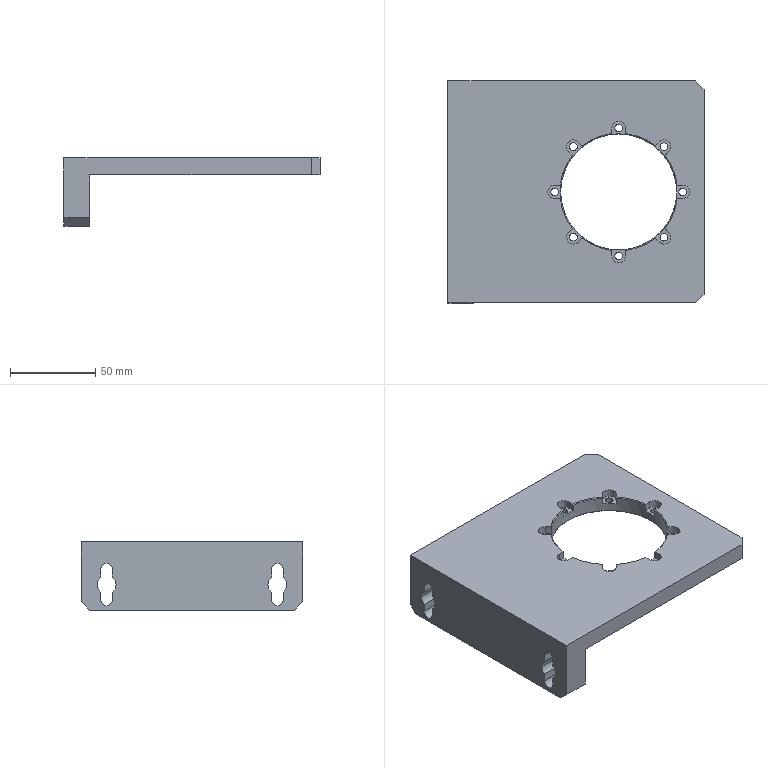NC program | NX | posted with a generic post | part box 150 x 130 x 40 mm
Whole program, first 1719 of 2019 lines:
N10 G17 G21 G94 G90
(FLOOR_WALL_COPY_COPY , TOOL : D80)
N12 T19 M6
N14 G54
N16 G17 G0 G90 X120. Y-64.997 B0. C0. S6500 M3
N18 G43 Z30. H19
N20 Z7.5
N22 G94 G1 Z4.5 F1500.
N24 X115.
N26 X-115.
N28 Y-55.429
N30 Y-15.999
N32 X115.
N34 Y33.
N36 X-115.
N38 X-120.
N40 Z7.5
N42 G0 Z30.
N44 X120. Y-64.997
N46 Z7.
N48 G1 Z4.
N50 X115.
N52 X-115.
N54 Y-55.429
N56 Y-15.999
N58 X115.
N60 Y33.
N62 X-115.
N64 X-120.
N66 Z7.
N68 G0 Z30.
N70 X120. Y-64.997
N72 Z6.5
N74 G1 Z3.5
N76 X115.
N78 X-115.
N80 Y-55.429
N82 Y-15.999
N84 X115.
N86 Y33.
N88 X-115.
N90 X-120.
N92 Z6.5
N94 G0 Z30.
N96 X120. Y-64.997
N98 Z6.
N100 G1 Z3.
N102 X115.
N104 X-115.
N106 Y-55.429
N108 Y-15.999
N110 X115.
N112 Y33.
N114 X-115.
N116 X-120.
N118 Z6.
N120 G0 Z30.
N122 X120. Y-64.997
N124 Z5.5
N126 G1 Z2.5
N128 X115.
N130 X-115.
N132 Y-55.429
N134 Y-15.999
N136 X115.
N138 Y33.
N140 X-115.
N142 X-120.
N144 Z5.5
N146 G0 Z30.
N148 X120. Y-64.997
N150 Z5.
N152 G1 Z2.
N154 X115.
N156 X-115.
N158 Y-55.429
N160 Y-15.999
N162 X115.
N164 Y33.
N166 X-115.
N168 X-120.
N170 Z5.
N172 G0 Z30.
N174 X120. Y-64.997
N176 Z4.5
N178 G1 Z1.5
N180 X115.
N182 X-115.
N184 Y-55.429
N186 Y-15.999
N188 X115.
N190 Y33.
N192 X-115.
N194 X-120.
N196 Z4.5
N198 G0 Z30.
N200 X120. Y-64.997
N202 Z4.
N204 G1 Z1.
N206 X115.
N208 X-115.
N210 Y-55.429
N212 Y-15.999
N214 X115.
N216 Y33.
N218 X-115.
N220 X-120.
N222 Z4.
N224 G0 Z30.
N226 X120. Y-64.997
N228 Z3.5
N230 G1 Z0.5
N232 X115.
N234 X-115.
N236 Y-55.429
N238 Y-15.999
N240 X115.
N242 Y33.
N244 X-115.
N246 X-120.
N248 Z3.5
N250 G0 Z30.
N252 X120. Y-64.997
N254 Z3.
N256 G1 Z0.
N258 X115.
N260 X-115.
N262 Y-55.429
N264 Y-15.999
N266 X115.
N268 Y33.
N270 X-115.
N272 X-120.
N274 Z3.
N276 G0 Z30.
N278 M5
(FLOOR_WALL , TOOL : D10)
N280 T15 M6
N282 G54
N284 G17 G0 G90 X80.5 Y73.5 B0. C0. S9500 M3
N286 G43 Z30. H15
N288 Z-11.95
N290 G94 G1 Z-14.95 F1000.
N292 Y70.5
N294 Y-70.142 F3000.
N296 G2 X80.142 Y-70.5 R0.358
N298 G1 X80.104
N300 G2 X79.704 Y-70.1 R0.4
N302 G1 Y70.142
N304 G3 X79.346 Y70.5 R0.358
N306 G1 X79.308
N308 G3 X78.908 Y70.1 R0.4
N310 G1 Y-70.142
N312 G2 X78.549 Y-70.5 R0.358
N314 G1 X78.511
N316 G2 X78.111 Y-70.1 R0.4
N318 G1 Y70.142
N320 G3 X77.753 Y70.5 R0.358
N322 G1 X77.715
N324 G3 X77.315 Y70.1 R0.4
N326 G1 Y-70.142
N328 G2 X76.957 Y-70.5 R0.358
N330 G1 X76.919
N332 G2 X76.519 Y-70.1 R0.4
N334 G1 Y70.142
N336 G3 X76.161 Y70.5 R0.358
N338 G1 X76.123
N340 G3 X75.723 Y70.1 R0.4
N342 G1 Y-70.142
N344 G2 X75.365 Y-70.5 R0.358
N346 G1 X75.327
N348 G2 X74.927 Y-70.1 R0.4
N350 G1 Y70.142
N352 G3 X74.568 Y70.5 R0.358
N354 G1 X74.531
N356 G3 X74.131 Y70.1 R0.4
N358 G1 Y-70.142
N360 G2 X73.772 Y-70.5 R0.358
N362 G1 X73.734
N364 G2 X73.334 Y-70.1 R0.4
N366 G1 Y70.142
N368 G3 X72.976 Y70.5 R0.358
N370 G1 X72.938
N372 G3 X72.538 Y70.1 R0.4
N374 G1 Y-70.142
N376 G2 X72.18 Y-70.5 R0.358
N378 G1 X72.142
N380 G2 X71.742 Y-70.1 R0.4
N382 G1 Y70.142
N384 G3 X71.384 Y70.5 R0.358
N386 G1 X71.346
N388 G3 X70.946 Y70.1 R0.4
N390 G1 Y-70.142
N392 G2 X70.588 Y-70.5 R0.358
N394 G1 X70.55
N396 G2 X70.15 Y-70.1 R0.4
N398 G1 Y70.142
N400 G3 X69.791 Y70.5 R0.358
N402 G1 X69.754
N404 G3 X69.354 Y70.1 R0.4
N406 G1 Y-70.142
N408 G2 X68.995 Y-70.5 R0.358
N410 G1 X68.957
N412 G2 X68.557 Y-70.1 R0.4
N414 G1 Y70.142
N416 G3 X68.199 Y70.5 R0.358
N418 G1 X68.161
N420 G3 X67.761 Y70.1 R0.4
N422 G1 Y-70.142
N424 G2 X67.403 Y-70.5 R0.358
N426 G1 X67.365
N428 G2 X66.965 Y-70.1 R0.4
N430 G1 Y70.142
N432 G3 X66.607 Y70.5 R0.358
N434 G1 X66.569
N436 G3 X66.169 Y70.1 R0.4
N438 G1 Y-70.142
N440 G2 X65.811 Y-70.5 R0.358
N442 G1 X65.773
N444 G2 X65.373 Y-70.1 R0.4
N446 G1 Y70.142
N448 G3 X65.014 Y70.5 R0.358
N450 G1 X64.976
N452 G3 X64.576 Y70.1 R0.4
N454 G1 Y-70.142
N456 G2 X64.218 Y-70.5 R0.358
N458 G1 X64.18
N460 G2 X63.78 Y-70.1 R0.4
N462 G1 Y70.142
N464 G3 X63.422 Y70.5 R0.358
N466 G1 X63.384
N468 G3 X62.984 Y70.1 R0.4
N470 G1 Y-70.142
N472 G2 X62.626 Y-70.5 R0.358
N474 G1 X62.588
N476 G2 X62.188 Y-70.1 R0.4
N478 G1 Y70.142
N480 G3 X61.83 Y70.5 R0.358
N482 G1 X61.792
N484 G3 X61.392 Y70.1 R0.4
N486 G1 Y-70.142
N488 G2 X61.033 Y-70.5 R0.358
N490 G1 X60.996
N492 G2 X60.596 Y-70.1 R0.4
N494 G1 Y70.142
N496 G3 X60.237 Y70.5 R0.358
N498 G1 X60.199
N500 G3 X59.799 Y70.1 R0.4
N502 G1 Y-70.142
N504 G2 X59.441 Y-70.5 R0.358
N506 G1 X59.403
N508 G2 X59.003 Y-70.1 R0.4
N510 G1 Y70.142
N512 G3 X58.645 Y70.5 R0.358
N514 G1 X58.607
N516 G3 X58.207 Y70.1 R0.4
N518 G1 Y-70.142
N520 G2 X57.849 Y-70.5 R0.358
N522 G1 X57.811
N524 G2 X57.411 Y-70.1 R0.4
N526 G1 Y70.142
N528 G3 X57.053 Y70.5 R0.358
N530 G1 X57.015
N532 G3 X56.615 Y70.1 R0.4
N534 G1 Y-70.142
N536 G2 X56.256 Y-70.5 R0.358
N538 G1 X56.219
N540 G2 X55.819 Y-70.1 R0.4
N542 G1 Y70.142
N544 G3 X55.46 Y70.5 R0.358
N546 G1 X55.422
N548 G3 X55.022 Y70.1 R0.4
N550 G1 Y-70.142
N552 G2 X54.664 Y-70.5 R0.358
N554 G1 X54.626
N556 G2 X54.226 Y-70.1 R0.4
N558 G1 Y70.142
N560 G3 X53.868 Y70.5 R0.358
N562 G1 X53.83
N564 G3 X53.43 Y70.1 R0.4
N566 G1 Y-70.142
N568 G2 X53.072 Y-70.5 R0.358
N570 G1 X53.034
N572 G2 X52.634 Y-70.1 R0.4
N574 G1 Y70.142
N576 G3 X52.276 Y70.5 R0.358
N578 G1 X52.238
N580 G3 X51.838 Y70.1 R0.4
N582 G1 Y-70.142
N584 G2 X51.479 Y-70.5 R0.358
N586 G1 X51.441
N588 G2 X51.041 Y-70.1 R0.4
N590 G1 Y70.142
N592 G3 X50.683 Y70.5 R0.358
N594 G1 X50.645
N596 G3 X50.245 Y70.1 R0.4
N598 G1 Y-70.142
N600 G2 X49.887 Y-70.5 R0.358
N602 G1 X49.849
N604 G2 X49.449 Y-70.1 R0.4
N606 G1 Y70.142
N608 G3 X49.091 Y70.5 R0.358
N610 G1 X49.053
N612 G3 X48.653 Y70.1 R0.4
N614 G1 Y-70.142
N616 G2 X48.295 Y-70.5 R0.358
N618 G1 X48.257
N620 G2 X47.857 Y-70.1 R0.4
N622 G1 Y70.142
N624 G3 X47.498 Y70.5 R0.358
N626 G1 X47.461
N628 G3 X47.061 Y70.1 R0.4
N630 G1 Y-70.142
N632 G2 X46.702 Y-70.5 R0.358
N634 G1 X46.664
N636 G2 X46.264 Y-70.1 R0.4
N638 G1 Y70.142
N640 G3 X45.906 Y70.5 R0.358
N642 G1 X45.868
N644 G3 X45.468 Y70.1 R0.4
N646 G1 Y-70.142
N648 G2 X45.11 Y-70.5 R0.358
N650 G1 X45.072
N652 G2 X44.672 Y-70.1 R0.4
N654 G1 Y70.142
N656 G3 X44.314 Y70.5 R0.358
N658 G1 X44.276
N660 G3 X43.876 Y70.1 R0.4
N662 G1 Y-70.142
N664 G2 X43.518 Y-70.5 R0.358
N666 G1 X43.48
N668 G2 X43.08 Y-70.1 R0.4
N670 G1 Y70.142
N672 G3 X42.721 Y70.5 R0.358
N674 G1 X42.684
N676 G3 X42.284 Y70.1 R0.4
N678 G1 Y-70.142
N680 G2 X41.925 Y-70.5 R0.358
N682 G1 X41.887
N684 G2 X41.487 Y-70.1 R0.4
N686 G1 Y70.142
N688 G3 X41.129 Y70.5 R0.358
N690 G1 X41.091
N692 G3 X40.691 Y70.1 R0.4
N694 G1 Y-70.142
N696 G2 X40.333 Y-70.5 R0.358
N698 G1 X40.295
N700 G2 X39.895 Y-70.1 R0.4
N702 G1 Y70.142
N704 G3 X39.537 Y70.5 R0.358
N706 G1 X39.499
N708 G3 X39.099 Y70.1 R0.4
N710 G1 Y-70.142
N712 G2 X38.741 Y-70.5 R0.358
N714 G1 X38.703
N716 G2 X38.303 Y-70.1 R0.4
N718 G1 Y70.142
N720 G3 X37.944 Y70.5 R0.358
N722 G1 X37.906
N724 G3 X37.506 Y70.1 R0.4
N726 G1 Y-70.142
N728 G2 X37.148 Y-70.5 R0.358
N730 G1 X37.11
N732 G2 X36.71 Y-70.1 R0.4
N734 G1 Y70.142
N736 G3 X36.352 Y70.5 R0.358
N738 G1 X36.314
N740 G3 X35.914 Y70.1 R0.4
N742 G1 Y-70.142
N744 G2 X35.556 Y-70.5 R0.358
N746 G1 X35.518
N748 G2 X35.118 Y-70.1 R0.4
N750 G1 Y70.142
N752 G3 X34.76 Y70.5 R0.358
N754 G1 X34.722
N756 G3 X34.322 Y70.1 R0.4
N758 G1 Y-70.142
N760 G2 X33.963 Y-70.5 R0.358
N762 G1 X33.926
N764 G2 X33.526 Y-70.1 R0.4
N766 G1 Y70.142
N768 G3 X33.167 Y70.5 R0.358
N770 G1 X33.129
N772 G3 X32.729 Y70.1 R0.4
N774 G1 Y-70.142
N776 G2 X32.371 Y-70.5 R0.358
N778 G1 X32.333
N780 G2 X31.933 Y-70.1 R0.4
N782 G1 Y70.142
N784 G3 X31.575 Y70.5 R0.358
N786 G1 X31.537
N788 G3 X31.137 Y70.1 R0.4
N790 G1 Y-70.142
N792 G2 X30.779 Y-70.5 R0.358
N794 G1 X30.741
N796 G2 X30.341 Y-70.1 R0.4
N798 G1 Y70.142
N800 G3 X29.983 Y70.5 R0.358
N802 G1 X29.945
N804 G3 X29.545 Y70.1 R0.4
N806 G1 Y-70.142
N808 G2 X29.186 Y-70.5 R0.358
N810 G1 X29.149
N812 G2 X28.749 Y-70.1 R0.4
N814 G1 Y70.142
N816 G3 X28.39 Y70.5 R0.358
N818 G1 X28.352
N820 G3 X27.952 Y70.1 R0.4
N822 G1 Y-70.142
N824 G2 X27.594 Y-70.5 R0.358
N826 G1 X27.556
N828 G2 X27.156 Y-70.1 R0.4
N830 G1 Y70.142
N832 G3 X26.798 Y70.5 R0.358
N834 G1 X26.76
N836 G3 X26.36 Y70.1 R0.4
N838 G1 Y-70.142
N840 G2 X26.002 Y-70.5 R0.358
N842 G1 X25.964
N844 G2 X25.564 Y-70.1 R0.4
N846 G1 Y70.142
N848 G3 X25.206 Y70.5 R0.358
N850 G1 X25.168
N852 G3 X24.768 Y70.1 R0.4
N854 G1 Y-70.142
N856 G2 X24.409 Y-70.5 R0.358
N858 G1 X24.371
N860 G2 X23.971 Y-70.1 R0.4
N862 G1 Y70.142
N864 G3 X23.613 Y70.5 R0.358
N866 G1 X23.575
N868 G3 X23.175 Y70.1 R0.4
N870 G1 Y-70.142
N872 G2 X22.817 Y-70.5 R0.358
N874 G1 X22.779
N876 G2 X22.379 Y-70.1 R0.4
N878 G1 Y70.142
N880 G3 X22.021 Y70.5 R0.358
N882 G1 X21.983
N884 G3 X21.583 Y70.1 R0.4
N886 G1 Y-70.142
N888 G2 X21.225 Y-70.5 R0.358
N890 G1 X21.187
N892 G2 X20.787 Y-70.1 R0.4
N894 G1 Y70.142
N896 G3 X20.428 Y70.5 R0.358
N898 G1 X20.391
N900 G3 X19.991 Y70.1 R0.4
N902 G1 Y-70.142
N904 G2 X19.632 Y-70.5 R0.358
N906 G1 X19.594
N908 G2 X19.194 Y-70.1 R0.4
N910 G1 Y70.142
N912 G3 X18.836 Y70.5 R0.358
N914 G1 X18.798
N916 G3 X18.398 Y70.1 R0.4
N918 G1 Y-70.142
N920 G2 X18.04 Y-70.5 R0.358
N922 G1 X18.002
N924 G2 X17.602 Y-70.1 R0.4
N926 G1 Y70.142
N928 G3 X17.244 Y70.5 R0.358
N930 G1 X17.206
N932 G3 X16.806 Y70.1 R0.4
N934 G1 Y-70.142
N936 G2 X16.448 Y-70.5 R0.358
N938 G1 X16.41
N940 G2 X16.01 Y-70.1 R0.4
N942 G1 Y70.142
N944 G3 X15.651 Y70.5 R0.358
N946 G1 X15.614
N948 G3 X15.214 Y70.1 R0.4
N950 G1 Y-70.142
N952 G2 X14.855 Y-70.5 R0.358
N954 G1 X14.817
N956 G2 X14.417 Y-70.1 R0.4
N958 G1 Y70.142
N960 G3 X14.059 Y70.5 R0.358
N962 G1 X14.021
N964 G3 X13.621 Y70.1 R0.4
N966 G1 Y-70.142
N968 G2 X13.263 Y-70.5 R0.358
N970 G1 X13.225
N972 G2 X12.825 Y-70.1 R0.4
N974 G1 Y70.142
N976 G3 X12.467 Y70.5 R0.358
N978 G1 X12.429
N980 G3 X12.029 Y70.1 R0.4
N982 G1 Y-70.142
N984 G2 X11.671 Y-70.5 R0.358
N986 G1 X11.633
N988 G2 X11.233 Y-70.1 R0.4
N990 G1 Y70.142
N992 G3 X10.874 Y70.5 R0.358
N994 G1 X10.836
N996 G3 X10.436 Y70.1 R0.4
N998 G1 Y-70.142
N1000 G2 X10.078 Y-70.5 R0.358
N1002 G1 X10.04
N1004 G2 X9.64 Y-70.1 R0.4
N1006 G1 Y70.142
N1008 G3 X9.282 Y70.5 R0.358
N1010 G1 X9.244
N1012 G3 X8.844 Y70.1 R0.4
N1014 G1 Y-70.142
N1016 G2 X8.486 Y-70.5 R0.358
N1018 G1 X8.448
N1020 G2 X8.048 Y-70.1 R0.4
N1022 G1 Y70.142
N1024 G3 X7.69 Y70.5 R0.358
N1026 G1 X7.652
N1028 G3 X7.252 Y70.1 R0.4
N1030 G1 Y-70.142
N1032 G2 X6.893 Y-70.5 R0.358
N1034 G1 X6.856
N1036 G2 X6.456 Y-70.1 R0.4
N1038 G1 Y70.142
N1040 G3 X6.097 Y70.5 R0.358
N1042 G1 X6.059
N1044 G3 X5.659 Y70.1 R0.4
N1046 G1 Y-70.142
N1048 G2 X5.301 Y-70.5 R0.358
N1050 G1 X5.263
N1052 G2 X4.863 Y-70.1 R0.4
N1054 G1 Y70.142
N1056 G3 X4.505 Y70.5 R0.358
N1058 G1 X4.467
N1060 G3 X4.067 Y70.1 R0.4
N1062 G1 Y-70.142
N1064 G2 X3.709 Y-70.5 R0.358
N1066 G1 X3.671
N1068 G2 X3.271 Y-70.1 R0.4
N1070 G1 Y70.142
N1072 G3 X2.913 Y70.5 R0.358
N1074 G1 X2.875
N1076 G3 X2.475 Y70.1 R0.4
N1078 G1 Y-70.142
N1080 G2 X2.116 Y-70.5 R0.358
N1082 G1 X2.079
N1084 G2 X1.679 Y-70.1 R0.4
N1086 G1 Y70.142
N1088 G3 X1.32 Y70.5 R0.358
N1090 G1 X1.282
N1092 G3 X0.882 Y70.1 R0.4
N1094 G1 Y-70.142
N1096 G2 X0.524 Y-70.5 R0.358
N1098 G1 X0.486
N1100 G2 X0.086 Y-70.1 R0.4
N1102 G1 Y70.142
N1104 G3 X-0.272 Y70.5 R0.358
N1106 G1 X-0.31
N1108 G3 X-0.71 Y70.1 R0.4
N1110 G1 Y-70.142
N1112 G2 X-1.068 Y-70.5 R0.358
N1114 G1 X-1.106
N1116 G2 X-1.506 Y-70.1 R0.4
N1118 G1 Y70.142
N1120 G3 X-1.864 Y70.5 R0.358
N1122 G1 X-1.902
N1124 G3 X-2.302 Y70.1 R0.4
N1126 G1 Y-70.142
N1128 G2 X-2.661 Y-70.5 R0.358
N1130 G1 X-2.699
N1132 G2 X-3.099 Y-70.1 R0.4
N1134 G1 Y70.142
N1136 G3 X-3.457 Y70.5 R0.358
N1138 G1 X-3.495
N1140 G3 X-3.895 Y70.1 R0.4
N1142 G1 Y-70.142
N1144 G2 X-4.253 Y-70.5 R0.358
N1146 G1 X-4.291
N1148 G2 X-4.691 Y-70.1 R0.4
N1150 G1 Y70.142
N1152 G3 X-5.049 Y70.5 R0.358
N1154 G1 X-5.087
N1156 G3 X-5.487 Y70.1 R0.4
N1158 G1 Y-70.142
N1160 G2 X-5.845 Y-70.5 R0.358
N1162 G1 X-5.883
N1164 G2 X-6.283 Y-70.1 R0.4
N1166 G1 Y70.142
N1168 G3 X-6.642 Y70.5 R0.358
N1170 G1 X-6.679
N1172 G3 X-7.079 Y70.1 R0.4
N1174 G1 Y-70.142
N1176 G2 X-7.438 Y-70.5 R0.358
N1178 G1 X-7.476
N1180 G2 X-7.876 Y-70.1 R0.4
N1182 G1 Y70.142
N1184 G3 X-8.234 Y70.5 R0.358
N1186 G1 X-8.272
N1188 G3 X-8.672 Y70.1 R0.4
N1190 G1 Y-70.142
N1192 G2 X-9.03 Y-70.5 R0.358
N1194 G1 X-9.068
N1196 G2 X-9.468 Y-70.1 R0.4
N1198 G1 Y70.142
N1200 G3 X-9.826 Y70.5 R0.358
N1202 G1 X-9.864
N1204 G3 X-10.264 Y70.1 R0.4
N1206 G1 Y-70.142
N1208 G2 X-10.622 Y-70.5 R0.358
N1210 G1 X-10.66
N1212 G2 X-11.06 Y-70.1 R0.4
N1214 G1 Y70.142
N1216 G3 X-11.419 Y70.5 R0.358
N1218 G1 X-11.456
N1220 G3 X-11.856 Y70.1 R0.4
N1222 G1 Y-70.142
N1224 G2 X-12.215 Y-70.5 R0.358
N1226 G1 X-12.253
N1228 G2 X-12.653 Y-70.1 R0.4
N1230 G1 Y70.142
N1232 G3 X-13.011 Y70.5 R0.358
N1234 G1 X-13.049
N1236 G3 X-13.449 Y70.1 R0.4
N1238 G1 Y-70.142
N1240 G2 X-13.807 Y-70.5 R0.358
N1242 G1 X-13.845
N1244 G2 X-14.245 Y-70.1 R0.4
N1246 G1 Y70.142
N1248 G3 X-14.603 Y70.5 R0.358
N1250 G1 X-14.641
N1252 G3 X-15.041 Y70.1 R0.4
N1254 G1 Y-70.142
N1256 G2 X-15.399 Y-70.5 R0.358
N1258 G1 X-15.437
N1260 G2 X-15.837 Y-70.1 R0.4
N1262 G1 Y70.142
N1264 G3 X-16.196 Y70.5 R0.358
N1266 G1 X-16.234
N1268 G3 X-16.634 Y70.1 R0.4
N1270 G1 Y-70.142
N1272 G2 X-16.992 Y-70.5 R0.358
N1274 G1 X-17.03
N1276 G2 X-17.43 Y-70.1 R0.4
N1278 G1 Y70.142
N1280 G3 X-17.788 Y70.5 R0.358
N1282 G1 X-17.826
N1284 G3 X-18.226 Y70.1 R0.4
N1286 G1 Y-70.142
N1288 G2 X-18.584 Y-70.5 R0.358
N1290 G1 X-18.622
N1292 G2 X-19.022 Y-70.1 R0.4
N1294 G1 Y70.142
N1296 G3 X-19.38 Y70.5 R0.358
N1298 G1 X-19.418
N1300 G3 X-19.818 Y70.1 R0.4
N1302 G1 Y-70.142
N1304 G2 X-20.177 Y-70.5 R0.358
N1306 G1 X-20.214
N1308 G2 X-20.614 Y-70.1 R0.4
N1310 G1 Y70.142
N1312 G3 X-20.973 Y70.5 R0.358
N1314 G1 X-21.011
N1316 G3 X-21.411 Y70.1 R0.4
N1318 G1 Y-70.142
N1320 G2 X-21.769 Y-70.5 R0.358
N1322 G1 X-21.807
N1324 G2 X-22.207 Y-70.1 R0.4
N1326 G1 Y70.142
N1328 G3 X-22.565 Y70.5 R0.358
N1330 G1 X-22.603
N1332 G3 X-23.003 Y70.1 R0.4
N1334 G1 Y-70.142
N1336 G2 X-23.361 Y-70.5 R0.358
N1338 G1 X-23.399
N1340 G2 X-23.799 Y-70.1 R0.4
N1342 G1 Y70.142
N1344 G3 X-24.157 Y70.5 R0.358
N1346 G1 X-24.195
N1348 G3 X-24.595 Y70.1 R0.4
N1350 G1 Y-70.142
N1352 G2 X-24.954 Y-70.5 R0.358
N1354 G1 X-24.991
N1356 G2 X-25.391 Y-70.1 R0.4
N1358 G1 Y70.142
N1360 G3 X-25.75 Y70.5 R0.358
N1362 G1 X-25.788
N1364 G3 X-26.188 Y70.1 R0.4
N1366 G1 Y-70.142
N1368 G2 X-26.546 Y-70.5 R0.358
N1370 G1 X-26.584
N1372 G2 X-26.984 Y-70.1 R0.4
N1374 G1 Y70.142
N1376 G3 X-27.342 Y70.5 R0.358
N1378 G1 X-27.38
N1380 G3 X-27.78 Y70.1 R0.4
N1382 G1 Y-70.142
N1384 G2 X-28.138 Y-70.5 R0.358
N1386 G1 X-28.176
N1388 G2 X-28.576 Y-70.1 R0.4
N1390 G1 Y70.142
N1392 G3 X-28.934 Y70.5 R0.358
N1394 G1 X-28.972
N1396 G3 X-29.372 Y70.1 R0.4
N1398 G1 Y-70.142
N1400 G2 X-29.731 Y-70.5 R0.358
N1402 G1 X-29.769
N1404 G2 X-30.169 Y-70.1 R0.4
N1406 G1 Y70.142
N1408 G3 X-30.527 Y70.5 R0.358
N1410 G1 X-30.565
N1412 G3 X-30.965 Y70.1 R0.4
N1414 G1 Y-70.142
N1416 G2 X-31.323 Y-70.5 R0.358
N1418 G1 X-31.361
N1420 G2 X-31.761 Y-70.1 R0.4
N1422 G1 Y70.142
N1424 G3 X-32.119 Y70.5 R0.358
N1426 G1 X-32.157
N1428 G3 X-32.557 Y70.1 R0.4
N1430 G1 Y-70.142
N1432 G2 X-32.915 Y-70.5 R0.358
N1434 G1 X-32.953
N1436 G2 X-33.353 Y-70.1 R0.4
N1438 G1 Y70.142
N1440 G3 X-33.712 Y70.5 R0.358
N1442 G1 X-33.749
N1444 G3 X-34.149 Y70.1 R0.4
N1446 G1 Y-70.142
N1448 G2 X-34.508 Y-70.5 R0.358
N1450 G1 X-34.546
N1452 G2 X-34.946 Y-70.1 R0.4
N1454 G1 Y70.142
N1456 G3 X-35.304 Y70.5 R0.358
N1458 G1 X-35.342
N1460 G3 X-35.742 Y70.1 R0.4
N1462 G1 Y-70.142
N1464 G2 X-36.1 Y-70.5 R0.358
N1466 G1 X-36.138
N1468 G2 X-36.538 Y-70.1 R0.4
N1470 G1 Y70.142
N1472 G3 X-36.896 Y70.5 R0.358
N1474 G1 X-36.934
N1476 G3 X-37.334 Y70.1 R0.4
N1478 G1 Y-70.142
N1480 G2 X-37.692 Y-70.5 R0.358
N1482 G1 X-37.73
N1484 G2 X-38.13 Y-70.1 R0.4
N1486 G1 Y70.142
N1488 G3 X-38.489 Y70.5 R0.358
N1490 G1 X-38.526
N1492 G3 X-38.926 Y70.1 R0.4
N1494 G1 Y-70.142
N1496 G2 X-39.285 Y-70.5 R0.358
N1498 G1 X-39.323
N1500 G2 X-39.723 Y-70.1 R0.4
N1502 G1 Y70.142
N1504 G3 X-40.081 Y70.5 R0.358
N1506 G1 X-40.119
N1508 G3 X-40.519 Y70.1 R0.4
N1510 G1 Y-70.142
N1512 G2 X-40.877 Y-70.5 R0.358
N1514 G1 X-40.915
N1516 G2 X-41.315 Y-70.1 R0.4
N1518 G1 Y70.142
N1520 G3 X-41.673 Y70.5 R0.358
N1522 G1 X-41.711
N1524 G3 X-42.111 Y70.1 R0.4
N1526 G1 Y-70.142
N1528 G2 X-42.469 Y-70.5 R0.358
N1530 G1 X-42.507
N1532 G2 X-42.907 Y-70.1 R0.4
N1534 G1 Y70.142
N1536 G3 X-43.266 Y70.5 R0.358
N1538 G1 X-43.304
N1540 G3 X-43.704 Y70.1 R0.4
N1542 G1 Y-70.142
N1544 G2 X-44.062 Y-70.5 R0.358
N1546 G1 X-44.1
N1548 G2 X-44.5 Y-70.1 R0.4
N1550 G1 Y70.142
N1552 G3 X-44.858 Y70.5 R0.358
N1554 G1 X-44.896
N1556 G3 X-45.296 Y70.1 R0.4
N1558 G1 Y-70.142
N1560 G2 X-45.654 Y-70.5 R0.358
N1562 G1 X-45.692
N1564 G2 X-46.092 Y-70.1 R0.4
N1566 G1 Y70.142
N1568 G3 X-46.45 Y70.5 R0.358
N1570 G1 X-46.488
N1572 G3 X-46.888 Y70.1 R0.4
N1574 G1 Y-70.142
N1576 G2 X-47.247 Y-70.5 R0.358
N1578 G1 X-47.284
N1580 G2 X-47.684 Y-70.1 R0.4
N1582 G1 Y70.142
N1584 G3 X-48.043 Y70.5 R0.358
N1586 G1 X-48.081
N1588 G3 X-48.481 Y70.1 R0.4
N1590 G1 Y-70.142
N1592 G2 X-48.839 Y-70.5 R0.358
N1594 G1 X-48.877
N1596 G2 X-49.277 Y-70.1 R0.4
N1598 G1 Y70.142
N1600 G3 X-49.635 Y70.5 R0.358
N1602 G1 X-49.673
N1604 G3 X-50.073 Y70.1 R0.4
N1606 G1 Y-70.142
N1608 G2 X-50.431 Y-70.5 R0.358
N1610 G1 X-50.469
N1612 G2 X-50.869 Y-70.1 R0.4
N1614 G1 Y70.142
N1616 G3 X-51.227 Y70.5 R0.358
N1618 G1 X-51.265
N1620 G3 X-51.665 Y70.1 R0.4
N1622 G1 Y-70.142
N1624 G2 X-52.024 Y-70.5 R0.358
N1626 G1 X-52.061
N1628 G2 X-52.461 Y-70.1 R0.4
N1630 G1 Y70.142
N1632 G3 X-52.82 Y70.5 R0.358
N1634 G1 X-52.858
N1636 G3 X-53.258 Y70.1 R0.4
N1638 G1 Y-70.142
N1640 G2 X-53.616 Y-70.5 R0.358
N1642 G1 X-53.654
N1644 G2 X-54.054 Y-70.1 R0.4
N1646 G1 Y70.142
N1648 G3 X-54.412 Y70.5 R0.358
N1650 G1 X-54.45
N1652 G3 X-54.85 Y70.1 R0.4
N1654 G1 Y-70.5
N1656 Y-73.5
N1658 Z-11.95
N1660 G0 Z30.
N1662 X80.5 Y73.5
N1664 Z-26.9
N1666 G1 Z-29.9 F1000.
N1668 Y70.5
N1670 Y-70.142 F3000.
N1672 G2 X80.142 Y-70.5 R0.358
N1674 G1 X80.104
N1676 G2 X79.704 Y-70.1 R0.4
N1678 G1 Y70.142
N1680 G3 X79.346 Y70.5 R0.358
N1682 G1 X79.308
N1684 G3 X78.908 Y70.1 R0.4
N1686 G1 Y-70.142
N1688 G2 X78.549 Y-70.5 R0.358
N1690 G1 X78.511
N1692 G2 X78.111 Y-70.1 R0.4
N1694 G1 Y70.142
N1696 G3 X77.753 Y70.5 R0.358
N1698 G1 X77.715
N1700 G3 X77.315 Y70.1 R0.4
N1702 G1 Y-70.142
N1704 G2 X76.957 Y-70.5 R0.358
N1706 G1 X76.919
N1708 G2 X76.519 Y-70.1 R0.4
N1710 G1 Y70.142
N1712 G3 X76.161 Y70.5 R0.358
N1714 G1 X76.123
N1716 G3 X75.723 Y70.1 R0.4
N1718 G1 Y-70.142
N1720 G2 X75.365 Y-70.5 R0.358
N1722 G1 X75.327
N1724 G2 X74.927 Y-70.1 R0.4
N1726 G1 Y70.142
N1728 G3 X74.568 Y70.5 R0.358
N1730 G1 X74.531
N1732 G3 X74.131 Y70.1 R0.4
N1734 G1 Y-70.142
N1736 G2 X73.772 Y-70.5 R0.358
N1738 G1 X73.734
N1740 G2 X73.334 Y-70.1 R0.4
N1742 G1 Y70.142
N1744 G3 X72.976 Y70.5 R0.358
N1746 G1 X72.938
N1748 G3 X72.538 Y70.1 R0.4
N1750 G1 Y-70.142
N1752 G2 X72.18 Y-70.5 R0.358
N1754 G1 X72.142
N1756 G2 X71.742 Y-70.1 R0.4
N1758 G1 Y70.142
N1760 G3 X71.384 Y70.5 R0.358
N1762 G1 X71.346
N1764 G3 X70.946 Y70.1 R0.4
N1766 G1 Y-70.142
N1768 G2 X70.588 Y-70.5 R0.358
N1770 G1 X70.55
N1772 G2 X70.15 Y-70.1 R0.4
N1774 G1 Y70.142
N1776 G3 X69.791 Y70.5 R0.358
N1778 G1 X69.754
N1780 G3 X69.354 Y70.1 R0.4
N1782 G1 Y-70.142
N1784 G2 X68.995 Y-70.5 R0.358
N1786 G1 X68.957
N1788 G2 X68.557 Y-70.1 R0.4
N1790 G1 Y70.142
N1792 G3 X68.199 Y70.5 R0.358
N1794 G1 X68.161
N1796 G3 X67.761 Y70.1 R0.4
N1798 G1 Y-70.142
N1800 G2 X67.403 Y-70.5 R0.358
N1802 G1 X67.365
N1804 G2 X66.965 Y-70.1 R0.4
N1806 G1 Y70.142
N1808 G3 X66.607 Y70.5 R0.358
N1810 G1 X66.569
N1812 G3 X66.169 Y70.1 R0.4
N1814 G1 Y-70.142
N1816 G2 X65.811 Y-70.5 R0.358
N1818 G1 X65.773
N1820 G2 X65.373 Y-70.1 R0.4
N1822 G1 Y70.142
N1824 G3 X65.014 Y70.5 R0.358
N1826 G1 X64.976
N1828 G3 X64.576 Y70.1 R0.4
N1830 G1 Y-70.142
N1832 G2 X64.218 Y-70.5 R0.358
N1834 G1 X64.18
N1836 G2 X63.78 Y-70.1 R0.4
N1838 G1 Y70.142
N1840 G3 X63.422 Y70.5 R0.358
N1842 G1 X63.384
N1844 G3 X62.984 Y70.1 R0.4
N1846 G1 Y-70.142
N1848 G2 X62.626 Y-70.5 R0.358
N1850 G1 X62.588
N1852 G2 X62.188 Y-70.1 R0.4
N1854 G1 Y70.142
N1856 G3 X61.83 Y70.5 R0.358
N1858 G1 X61.792
N1860 G3 X61.392 Y70.1 R0.4
N1862 G1 Y-70.142
N1864 G2 X61.033 Y-70.5 R0.358
N1866 G1 X60.996
N1868 G2 X60.596 Y-70.1 R0.4
N1870 G1 Y70.142
N1872 G3 X60.237 Y70.5 R0.358
N1874 G1 X60.199
N1876 G3 X59.799 Y70.1 R0.4
N1878 G1 Y-70.142
N1880 G2 X59.441 Y-70.5 R0.358
N1882 G1 X59.403
N1884 G2 X59.003 Y-70.1 R0.4
N1886 G1 Y70.142
N1888 G3 X58.645 Y70.5 R0.358
N1890 G1 X58.607
N1892 G3 X58.207 Y70.1 R0.4
N1894 G1 Y-70.142
N1896 G2 X57.849 Y-70.5 R0.358
N1898 G1 X57.811
N1900 G2 X57.411 Y-70.1 R0.4
N1902 G1 Y70.142
N1904 G3 X57.053 Y70.5 R0.358
N1906 G1 X57.015
N1908 G3 X56.615 Y70.1 R0.4
N1910 G1 Y-70.142
N1912 G2 X56.256 Y-70.5 R0.358
N1914 G1 X56.219
N1916 G2 X55.819 Y-70.1 R0.4
N1918 G1 Y70.142
N1920 G3 X55.46 Y70.5 R0.358
N1922 G1 X55.422
N1924 G3 X55.022 Y70.1 R0.4
N1926 G1 Y-70.142
N1928 G2 X54.664 Y-70.5 R0.358
N1930 G1 X54.626
N1932 G2 X54.226 Y-70.1 R0.4
N1934 G1 Y70.142
N1936 G3 X53.868 Y70.5 R0.358
N1938 G1 X53.83
N1940 G3 X53.43 Y70.1 R0.4
N1942 G1 Y-70.142
N1944 G2 X53.072 Y-70.5 R0.358
N1946 G1 X53.034
N1948 G2 X52.634 Y-70.1 R0.4
N1950 G1 Y70.142
N1952 G3 X52.276 Y70.5 R0.358
N1954 G1 X52.238
N1956 G3 X51.838 Y70.1 R0.4
N1958 G1 Y-70.142
N1960 G2 X51.479 Y-70.5 R0.358
N1962 G1 X51.441
N1964 G2 X51.041 Y-70.1 R0.4
N1966 G1 Y70.142
N1968 G3 X50.683 Y70.5 R0.358
N1970 G1 X50.645
N1972 G3 X50.245 Y70.1 R0.4
N1974 G1 Y-70.142
N1976 G2 X49.887 Y-70.5 R0.358
N1978 G1 X49.849
N1980 G2 X49.449 Y-70.1 R0.4
N1982 G1 Y70.142
N1984 G3 X49.091 Y70.5 R0.358
N1986 G1 X49.053
N1988 G3 X48.653 Y70.1 R0.4
N1990 G1 Y-70.142
N1992 G2 X48.295 Y-70.5 R0.358
N1994 G1 X48.257
N1996 G2 X47.857 Y-70.1 R0.4
N1998 G1 Y70.142
N2000 G3 X47.498 Y70.5 R0.358
N2002 G1 X47.461
N2004 G3 X47.061 Y70.1 R0.4
N2006 G1 Y-70.142
N2008 G2 X46.702 Y-70.5 R0.358
N2010 G1 X46.664
N2012 G2 X46.264 Y-70.1 R0.4
N2014 G1 Y70.142
N2016 G3 X45.906 Y70.5 R0.358
N2018 G1 X45.868
N2020 G3 X45.468 Y70.1 R0.4
N2022 G1 Y-70.142
N2024 G2 X45.11 Y-70.5 R0.358
N2026 G1 X45.072
N2028 G2 X44.672 Y-70.1 R0.4
N2030 G1 Y70.142
N2032 G3 X44.314 Y70.5 R0.358
N2034 G1 X44.276
N2036 G3 X43.876 Y70.1 R0.4
N2038 G1 Y-70.142
N2040 G2 X43.518 Y-70.5 R0.358
N2042 G1 X43.48
N2044 G2 X43.08 Y-70.1 R0.4
N2046 G1 Y70.142
N2048 G3 X42.721 Y70.5 R0.358
N2050 G1 X42.684
N2052 G3 X42.284 Y70.1 R0.4
N2054 G1 Y-70.142
N2056 G2 X41.925 Y-70.5 R0.358
N2058 G1 X41.887
N2060 G2 X41.487 Y-70.1 R0.4
N2062 G1 Y70.142
N2064 G3 X41.129 Y70.5 R0.358
N2066 G1 X41.091
N2068 G3 X40.691 Y70.1 R0.4
N2070 G1 Y-70.142
N2072 G2 X40.333 Y-70.5 R0.358
N2074 G1 X40.295
N2076 G2 X39.895 Y-70.1 R0.4
N2078 G1 Y70.142
N2080 G3 X39.537 Y70.5 R0.358
N2082 G1 X39.499
N2084 G3 X39.099 Y70.1 R0.4
N2086 G1 Y-70.142
N2088 G2 X38.741 Y-70.5 R0.358
N2090 G1 X38.703
N2092 G2 X38.303 Y-70.1 R0.4
N2094 G1 Y70.142
N2096 G3 X37.944 Y70.5 R0.358
N2098 G1 X37.906
N2100 G3 X37.506 Y70.1 R0.4
N2102 G1 Y-70.142
N2104 G2 X37.148 Y-70.5 R0.358
N2106 G1 X37.11
N2108 G2 X36.71 Y-70.1 R0.4
N2110 G1 Y70.142
N2112 G3 X36.352 Y70.5 R0.358
N2114 G1 X36.314
N2116 G3 X35.914 Y70.1 R0.4
N2118 G1 Y-70.142
N2120 G2 X35.556 Y-70.5 R0.358
N2122 G1 X35.518
N2124 G2 X35.118 Y-70.1 R0.4
N2126 G1 Y70.142
N2128 G3 X34.76 Y70.5 R0.358
N2130 G1 X34.722
N2132 G3 X34.322 Y70.1 R0.4
N2134 G1 Y-70.142
N2136 G2 X33.963 Y-70.5 R0.358
N2138 G1 X33.926
N2140 G2 X33.526 Y-70.1 R0.4
N2142 G1 Y70.142
N2144 G3 X33.167 Y70.5 R0.358
N2146 G1 X33.129
N2148 G3 X32.729 Y70.1 R0.4
N2150 G1 Y-70.142
N2152 G2 X32.371 Y-70.5 R0.358
N2154 G1 X32.333
N2156 G2 X31.933 Y-70.1 R0.4
N2158 G1 Y70.142
N2160 G3 X31.575 Y70.5 R0.358
N2162 G1 X31.537
N2164 G3 X31.137 Y70.1 R0.4
N2166 G1 Y-70.142
N2168 G2 X30.779 Y-70.5 R0.358
N2170 G1 X30.741
N2172 G2 X30.341 Y-70.1 R0.4
N2174 G1 Y70.142
N2176 G3 X29.983 Y70.5 R0.358
N2178 G1 X29.945
N2180 G3 X29.545 Y70.1 R0.4
N2182 G1 Y-70.142
N2184 G2 X29.186 Y-70.5 R0.358
N2186 G1 X29.149
N2188 G2 X28.749 Y-70.1 R0.4
N2190 G1 Y70.142
N2192 G3 X28.39 Y70.5 R0.358
N2194 G1 X28.352
N2196 G3 X27.952 Y70.1 R0.4
N2198 G1 Y-70.142
N2200 G2 X27.594 Y-70.5 R0.358
N2202 G1 X27.556
N2204 G2 X27.156 Y-70.1 R0.4
N2206 G1 Y70.142
N2208 G3 X26.798 Y70.5 R0.358
N2210 G1 X26.76
N2212 G3 X26.36 Y70.1 R0.4
N2214 G1 Y-70.142
N2216 G2 X26.002 Y-70.5 R0.358
N2218 G1 X25.964
N2220 G2 X25.564 Y-70.1 R0.4
N2222 G1 Y70.142
N2224 G3 X25.206 Y70.5 R0.358
N2226 G1 X25.168
N2228 G3 X24.768 Y70.1 R0.4
N2230 G1 Y-70.142
N2232 G2 X24.409 Y-70.5 R0.358
N2234 G1 X24.371
N2236 G2 X23.971 Y-70.1 R0.4
N2238 G1 Y70.142
N2240 G3 X23.613 Y70.5 R0.358
N2242 G1 X23.575
N2244 G3 X23.175 Y70.1 R0.4
N2246 G1 Y-70.142
N2248 G2 X22.817 Y-70.5 R0.358
N2250 G1 X22.779
N2252 G2 X22.379 Y-70.1 R0.4
N2254 G1 Y70.142
N2256 G3 X22.021 Y70.5 R0.358
N2258 G1 X21.983
N2260 G3 X21.583 Y70.1 R0.4
N2262 G1 Y-70.142
N2264 G2 X21.225 Y-70.5 R0.358
N2266 G1 X21.187
N2268 G2 X20.787 Y-70.1 R0.4
N2270 G1 Y70.142
N2272 G3 X20.428 Y70.5 R0.358
N2274 G1 X20.391
N2276 G3 X19.991 Y70.1 R0.4
N2278 G1 Y-70.142
N2280 G2 X19.632 Y-70.5 R0.358
N2282 G1 X19.594
N2284 G2 X19.194 Y-70.1 R0.4
N2286 G1 Y70.142
N2288 G3 X18.836 Y70.5 R0.358
N2290 G1 X18.798
N2292 G3 X18.398 Y70.1 R0.4
N2294 G1 Y-70.142
N2296 G2 X18.04 Y-70.5 R0.358
N2298 G1 X18.002
N2300 G2 X17.602 Y-70.1 R0.4
N2302 G1 Y70.142
N2304 G3 X17.244 Y70.5 R0.358
N2306 G1 X17.206
N2308 G3 X16.806 Y70.1 R0.4
N2310 G1 Y-70.142
N2312 G2 X16.448 Y-70.5 R0.358
N2314 G1 X16.41
N2316 G2 X16.01 Y-70.1 R0.4
N2318 G1 Y70.142
N2320 G3 X15.651 Y70.5 R0.358
N2322 G1 X15.614
N2324 G3 X15.214 Y70.1 R0.4
N2326 G1 Y-70.142
N2328 G2 X14.855 Y-70.5 R0.358
N2330 G1 X14.817
N2332 G2 X14.417 Y-70.1 R0.4
N2334 G1 Y70.142
N2336 G3 X14.059 Y70.5 R0.358
N2338 G1 X14.021
N2340 G3 X13.621 Y70.1 R0.4
N2342 G1 Y-70.142
N2344 G2 X13.263 Y-70.5 R0.358
N2346 G1 X13.225
N2348 G2 X12.825 Y-70.1 R0.4
N2350 G1 Y70.142
N2352 G3 X12.467 Y70.5 R0.358
N2354 G1 X12.429
N2356 G3 X12.029 Y70.1 R0.4
N2358 G1 Y-70.142
N2360 G2 X11.671 Y-70.5 R0.358
N2362 G1 X11.633
N2364 G2 X11.233 Y-70.1 R0.4
N2366 G1 Y70.142
N2368 G3 X10.874 Y70.5 R0.358
N2370 G1 X10.836
N2372 G3 X10.436 Y70.1 R0.4
N2374 G1 Y-70.142
N2376 G2 X10.078 Y-70.5 R0.358
N2378 G1 X10.04
N2380 G2 X9.64 Y-70.1 R0.4
N2382 G1 Y70.142
N2384 G3 X9.282 Y70.5 R0.358
N2386 G1 X9.244
N2388 G3 X8.844 Y70.1 R0.4
N2390 G1 Y-70.142
N2392 G2 X8.486 Y-70.5 R0.358
N2394 G1 X8.448
N2396 G2 X8.048 Y-70.1 R0.4
N2398 G1 Y70.142
N2400 G3 X7.69 Y70.5 R0.358
N2402 G1 X7.652
N2404 G3 X7.252 Y70.1 R0.4
N2406 G1 Y-70.142
N2408 G2 X6.893 Y-70.5 R0.358
N2410 G1 X6.856
N2412 G2 X6.456 Y-70.1 R0.4
N2414 G1 Y70.142
N2416 G3 X6.097 Y70.5 R0.358
N2418 G1 X6.059
N2420 G3 X5.659 Y70.1 R0.4
N2422 G1 Y-70.142
N2424 G2 X5.301 Y-70.5 R0.358
N2426 G1 X5.263
N2428 G2 X4.863 Y-70.1 R0.4
N2430 G1 Y70.142
N2432 G3 X4.505 Y70.5 R0.358
N2434 G1 X4.467
N2436 G3 X4.067 Y70.1 R0.4
N2438 G1 Y-70.142
N2440 G2 X3.709 Y-70.5 R0.358
N2442 G1 X3.671
N2444 G2 X3.271 Y-70.1 R0.4
N2446 G1 Y70.142
N2448 G3 X2.913 Y70.5 R0.358
N2450 G1 X2.875
N2452 G3 X2.475 Y70.1 R0.4
N2454 G1 Y-70.142
N2456 G2 X2.116 Y-70.5 R0.358
N2458 G1 X2.079
N2460 G2 X1.679 Y-70.1 R0.4
N2462 G1 Y70.142
N2464 G3 X1.32 Y70.5 R0.358
N2466 G1 X1.282
N2468 G3 X0.882 Y70.1 R0.4
N2470 G1 Y-70.142
N2472 G2 X0.524 Y-70.5 R0.358
N2474 G1 X0.486
N2476 G2 X0.086 Y-70.1 R0.4
N2478 G1 Y70.142
N2480 G3 X-0.272 Y70.5 R0.358
N2482 G1 X-0.31
N2484 G3 X-0.71 Y70.1 R0.4
N2486 G1 Y-70.142
N2488 G2 X-1.068 Y-70.5 R0.358
N2490 G1 X-1.106
N2492 G2 X-1.506 Y-70.1 R0.4
N2494 G1 Y70.142
N2496 G3 X-1.864 Y70.5 R0.358
N2498 G1 X-1.902
N2500 G3 X-2.302 Y70.1 R0.4
N2502 G1 Y-70.142
N2504 G2 X-2.661 Y-70.5 R0.358
N2506 G1 X-2.699
N2508 G2 X-3.099 Y-70.1 R0.4
N2510 G1 Y70.142
N2512 G3 X-3.457 Y70.5 R0.358
N2514 G1 X-3.495
N2516 G3 X-3.895 Y70.1 R0.4
N2518 G1 Y-70.142
N2520 G2 X-4.253 Y-70.5 R0.358
N2522 G1 X-4.291
N2524 G2 X-4.691 Y-70.1 R0.4
N2526 G1 Y70.142
N2528 G3 X-5.049 Y70.5 R0.358
N2530 G1 X-5.087
N2532 G3 X-5.487 Y70.1 R0.4
N2534 G1 Y-70.142
N2536 G2 X-5.845 Y-70.5 R0.358
N2538 G1 X-5.883
N2540 G2 X-6.283 Y-70.1 R0.4
N2542 G1 Y70.142
N2544 G3 X-6.642 Y70.5 R0.358
N2546 G1 X-6.679
N2548 G3 X-7.079 Y70.1 R0.4
N2550 G1 Y-70.142
N2552 G2 X-7.438 Y-70.5 R0.358
N2554 G1 X-7.476
N2556 G2 X-7.876 Y-70.1 R0.4
N2558 G1 Y70.142
N2560 G3 X-8.234 Y70.5 R0.358
N2562 G1 X-8.272
N2564 G3 X-8.672 Y70.1 R0.4
N2566 G1 Y-70.142
N2568 G2 X-9.03 Y-70.5 R0.358
N2570 G1 X-9.068
N2572 G2 X-9.468 Y-70.1 R0.4
N2574 G1 Y70.142
N2576 G3 X-9.826 Y70.5 R0.358
N2578 G1 X-9.864
N2580 G3 X-10.264 Y70.1 R0.4
N2582 G1 Y-70.142
N2584 G2 X-10.622 Y-70.5 R0.358
N2586 G1 X-10.66
N2588 G2 X-11.06 Y-70.1 R0.4
N2590 G1 Y70.142
N2592 G3 X-11.419 Y70.5 R0.358
N2594 G1 X-11.456
N2596 G3 X-11.856 Y70.1 R0.4
N2598 G1 Y-70.142
N2600 G2 X-12.215 Y-70.5 R0.358
N2602 G1 X-12.253
N2604 G2 X-12.653 Y-70.1 R0.4
N2606 G1 Y70.142
N2608 G3 X-13.011 Y70.5 R0.358
N2610 G1 X-13.049
N2612 G3 X-13.449 Y70.1 R0.4
N2614 G1 Y-70.142
N2616 G2 X-13.807 Y-70.5 R0.358
N2618 G1 X-13.845
N2620 G2 X-14.245 Y-70.1 R0.4
N2622 G1 Y70.142
N2624 G3 X-14.603 Y70.5 R0.358
N2626 G1 X-14.641
N2628 G3 X-15.041 Y70.1 R0.4
N2630 G1 Y-70.142
N2632 G2 X-15.399 Y-70.5 R0.358
N2634 G1 X-15.437
N2636 G2 X-15.837 Y-70.1 R0.4
N2638 G1 Y70.142
N2640 G3 X-16.196 Y70.5 R0.358
N2642 G1 X-16.234
N2644 G3 X-16.634 Y70.1 R0.4
N2646 G1 Y-70.142
N2648 G2 X-16.992 Y-70.5 R0.358
N2650 G1 X-17.03
N2652 G2 X-17.43 Y-70.1 R0.4
N2654 G1 Y70.142
N2656 G3 X-17.788 Y70.5 R0.358
N2658 G1 X-17.826
N2660 G3 X-18.226 Y70.1 R0.4
N2662 G1 Y-70.142
N2664 G2 X-18.584 Y-70.5 R0.358
N2666 G1 X-18.622
N2668 G2 X-19.022 Y-70.1 R0.4
N2670 G1 Y70.142
N2672 G3 X-19.38 Y70.5 R0.358
N2674 G1 X-19.418
N2676 G3 X-19.818 Y70.1 R0.4
N2678 G1 Y-70.142
N2680 G2 X-20.177 Y-70.5 R0.358
N2682 G1 X-20.214
N2684 G2 X-20.614 Y-70.1 R0.4
N2686 G1 Y70.142
N2688 G3 X-20.973 Y70.5 R0.358
N2690 G1 X-21.011
N2692 G3 X-21.411 Y70.1 R0.4
N2694 G1 Y-70.142
N2696 G2 X-21.769 Y-70.5 R0.358
N2698 G1 X-21.807
N2700 G2 X-22.207 Y-70.1 R0.4
N2702 G1 Y70.142
N2704 G3 X-22.565 Y70.5 R0.358
N2706 G1 X-22.603
N2708 G3 X-23.003 Y70.1 R0.4
N2710 G1 Y-70.142
N2712 G2 X-23.361 Y-70.5 R0.358
N2714 G1 X-23.399
N2716 G2 X-23.799 Y-70.1 R0.4
N2718 G1 Y70.142
N2720 G3 X-24.157 Y70.5 R0.358
N2722 G1 X-24.195
N2724 G3 X-24.595 Y70.1 R0.4
N2726 G1 Y-70.142
N2728 G2 X-24.954 Y-70.5 R0.358
N2730 G1 X-24.991
N2732 G2 X-25.391 Y-70.1 R0.4
N2734 G1 Y70.142
N2736 G3 X-25.75 Y70.5 R0.358
N2738 G1 X-25.788
N2740 G3 X-26.188 Y70.1 R0.4
N2742 G1 Y-70.142
N2744 G2 X-26.546 Y-70.5 R0.358
N2746 G1 X-26.584
N2748 G2 X-26.984 Y-70.1 R0.4
N2750 G1 Y70.142
N2752 G3 X-27.342 Y70.5 R0.358
N2754 G1 X-27.38
N2756 G3 X-27.78 Y70.1 R0.4
N2758 G1 Y-70.142
N2760 G2 X-28.138 Y-70.5 R0.358
N2762 G1 X-28.176
N2764 G2 X-28.576 Y-70.1 R0.4
N2766 G1 Y70.142
N2768 G3 X-28.934 Y70.5 R0.358
N2770 G1 X-28.972
N2772 G3 X-29.372 Y70.1 R0.4
N2774 G1 Y-70.142
N2776 G2 X-29.731 Y-70.5 R0.358
N2778 G1 X-29.769
N2780 G2 X-30.169 Y-70.1 R0.4
N2782 G1 Y70.142
N2784 G3 X-30.527 Y70.5 R0.358
N2786 G1 X-30.565
N2788 G3 X-30.965 Y70.1 R0.4
N2790 G1 Y-70.142
N2792 G2 X-31.323 Y-70.5 R0.358
N2794 G1 X-31.361
N2796 G2 X-31.761 Y-70.1 R0.4
N2798 G1 Y70.142
N2800 G3 X-32.119 Y70.5 R0.358
N2802 G1 X-32.157
N2804 G3 X-32.557 Y70.1 R0.4
N2806 G1 Y-70.142
N2808 G2 X-32.915 Y-70.5 R0.358
N2810 G1 X-32.953
N2812 G2 X-33.353 Y-70.1 R0.4
N2814 G1 Y70.142
N2816 G3 X-33.712 Y70.5 R0.358
N2818 G1 X-33.749
N2820 G3 X-34.149 Y70.1 R0.4
N2822 G1 Y-70.142
N2824 G2 X-34.508 Y-70.5 R0.358
N2826 G1 X-34.546
N2828 G2 X-34.946 Y-70.1 R0.4
N2830 G1 Y70.142
N2832 G3 X-35.304 Y70.5 R0.358
N2834 G1 X-35.342
N2836 G3 X-35.742 Y70.1 R0.4
N2838 G1 Y-70.142
N2840 G2 X-36.1 Y-70.5 R0.358
N2842 G1 X-36.138
N2844 G2 X-36.538 Y-70.1 R0.4
N2846 G1 Y70.142
N2848 G3 X-36.896 Y70.5 R0.358
N2850 G1 X-36.934
N2852 G3 X-37.334 Y70.1 R0.4
N2854 G1 Y-70.142
N2856 G2 X-37.692 Y-70.5 R0.358
N2858 G1 X-37.73
N2860 G2 X-38.13 Y-70.1 R0.4
N2862 G1 Y70.142
N2864 G3 X-38.489 Y70.5 R0.358
N2866 G1 X-38.526
N2868 G3 X-38.926 Y70.1 R0.4
N2870 G1 Y-70.142
N2872 G2 X-39.285 Y-70.5 R0.358
N2874 G1 X-39.323
N2876 G2 X-39.723 Y-70.1 R0.4
N2878 G1 Y70.142
N2880 G3 X-40.081 Y70.5 R0.358
N2882 G1 X-40.119
N2884 G3 X-40.519 Y70.1 R0.4
N2886 G1 Y-70.142
N2888 G2 X-40.877 Y-70.5 R0.358
N2890 G1 X-40.915
N2892 G2 X-41.315 Y-70.1 R0.4
N2894 G1 Y70.142
N2896 G3 X-41.673 Y70.5 R0.358
N2898 G1 X-41.711
N2900 G3 X-42.111 Y70.1 R0.4
N2902 G1 Y-70.142
N2904 G2 X-42.469 Y-70.5 R0.358
N2906 G1 X-42.507
N2908 G2 X-42.907 Y-70.1 R0.4
N2910 G1 Y70.142
N2912 G3 X-43.266 Y70.5 R0.358
N2914 G1 X-43.304
N2916 G3 X-43.704 Y70.1 R0.4
N2918 G1 Y-70.142
N2920 G2 X-44.062 Y-70.5 R0.358
N2922 G1 X-44.1
N2924 G2 X-44.5 Y-70.1 R0.4
N2926 G1 Y70.142
N2928 G3 X-44.858 Y70.5 R0.358
N2930 G1 X-44.896
N2932 G3 X-45.296 Y70.1 R0.4
N2934 G1 Y-70.142
N2936 G2 X-45.654 Y-70.5 R0.358
N2938 G1 X-45.692
N2940 G2 X-46.092 Y-70.1 R0.4
N2942 G1 Y70.142
N2944 G3 X-46.45 Y70.5 R0.358
N2946 G1 X-46.488
N2948 G3 X-46.888 Y70.1 R0.4
N2950 G1 Y-70.142
N2952 G2 X-47.247 Y-70.5 R0.358
N2954 G1 X-47.284
N2956 G2 X-47.684 Y-70.1 R0.4
N2958 G1 Y70.142
N2960 G3 X-48.043 Y70.5 R0.358
N2962 G1 X-48.081
N2964 G3 X-48.481 Y70.1 R0.4
N2966 G1 Y-70.142
N2968 G2 X-48.839 Y-70.5 R0.358
N2970 G1 X-48.877
N2972 G2 X-49.277 Y-70.1 R0.4
N2974 G1 Y70.142
N2976 G3 X-49.635 Y70.5 R0.358
N2978 G1 X-49.673
N2980 G3 X-50.073 Y70.1 R0.4
N2982 G1 Y-70.142
N2984 G2 X-50.431 Y-70.5 R0.358
N2986 G1 X-50.469
N2988 G2 X-50.869 Y-70.1 R0.4
N2990 G1 Y70.142
N2992 G3 X-51.227 Y70.5 R0.358
N2994 G1 X-51.265
N2996 G3 X-51.665 Y70.1 R0.4
N2998 G1 Y-70.142
N3000 G2 X-52.024 Y-70.5 R0.358
N3002 G1 X-52.061
N3004 G2 X-52.461 Y-70.1 R0.4
N3006 G1 Y70.142
N3008 G3 X-52.82 Y70.5 R0.358
N3010 G1 X-52.858
N3012 G3 X-53.258 Y70.1 R0.4
N3014 G1 Y-70.142
N3016 G2 X-53.616 Y-70.5 R0.358
N3018 G1 X-53.654
N3020 G2 X-54.054 Y-70.1 R0.4
N3022 G1 Y70.142
N3024 G3 X-54.412 Y70.5 R0.358
N3026 G1 X-54.45
N3028 G3 X-54.85 Y70.1 R0.4
N3030 G1 Y-70.5
N3032 Y-73.5
N3034 Z-26.9
N3036 G0 Z30.
N3038 M5
(FLOOR_WALL_COPY_1 , TOOL : D10JING)
N3040 T14 M6
N3042 G54
N3044 G17 G0 G90 X-55. Y73. B0. C0. S9500 M3
N3046 G43 Z30. H14
N3048 Z-11.95
N3050 G94 G1 Z-14.95 F1000.
N3052 Y70.
N3054 Y-70. F1200.
N3056 Y-73.
N3058 Z-11.95
N3060 G0 Z30.
N3062 Y73.
N3064 Z-26.9
N3066 G1 Z-29.9 F1000.
N3068 Y70.
N3070 Y-70. F1200.
N3072 Y-73.
N3074 Z-26.9
N3076 G0 Z30.
(FLOOR_WALL_COPY_1_COPY , TOOL : D10JING)
N3078 X80. Y73.
N3080 Z-27.
N3082 G1 Z-30. F1000.
N3084 Y70.
N3086 Y-67.758 F1200.
N3088 G2 X77.758 Y-70. R2.242
N3090 G1 X77.519
N3092 G2 X75.019 Y-67.5 R2.5
N3094 G1 Y67.758
N3096 G3 X72.777 Y70. R2.242
N3098 G1 X72.537
N3100 G3 X70.037 Y67.5 R2.5
N3102 G1 Y-67.758
N3104 G2 X67.795 Y-70. R2.242
N3106 G1 X67.556
N3108 G2 X65.056 Y-67.5 R2.5
N3110 G1 Y67.758
N3112 G3 X62.814 Y70. R2.242
N3114 G1 X62.574
N3116 G3 X60.074 Y67.5 R2.5
N3118 G1 Y-67.758
N3120 G2 X57.832 Y-70. R2.242
N3122 G1 X57.593
N3124 G2 X55.093 Y-67.5 R2.5
N3126 G1 Y67.758
N3128 G3 X52.851 Y70. R2.242
N3130 G1 X52.611
N3132 G3 X50.111 Y67.5 R2.5
N3134 G1 Y-67.758
N3136 G2 X47.869 Y-70. R2.242
N3138 G1 X47.63
N3140 G2 X45.13 Y-67.5 R2.5
N3142 G1 Y67.758
N3144 G3 X42.888 Y70. R2.242
N3146 G1 X42.648
N3148 G3 X40.148 Y67.5 R2.5
N3150 G1 Y-67.758
N3152 G2 X37.906 Y-70. R2.242
N3154 G1 X37.667
N3156 G2 X35.167 Y-67.5 R2.5
N3158 G1 Y67.758
N3160 G3 X32.925 Y70. R2.242
N3162 G1 X32.685
N3164 G3 X30.185 Y67.5 R2.5
N3166 G1 Y-67.758
N3168 G2 X27.944 Y-70. R2.242
N3170 G1 X27.704
N3172 G2 X25.204 Y-67.5 R2.5
N3174 G1 Y67.758
N3176 G3 X22.962 Y70. R2.242
N3178 G1 X22.722
N3180 G3 X20.222 Y67.5 R2.5
N3182 G1 Y-67.758
N3184 G2 X17.981 Y-70. R2.242
N3186 G1 X17.741
N3188 G2 X15.241 Y-67.5 R2.5
N3190 G1 Y67.758
N3192 G3 X12.999 Y70. R2.242
N3194 G1 X12.759
N3196 G3 X10.259 Y67.5 R2.5
N3198 G1 Y-67.758
N3200 G2 X8.018 Y-70. R2.242
N3202 G1 X7.778
N3204 G2 X5.278 Y-67.5 R2.5
N3206 G1 Y67.509
N3208 G3 X2.787 Y70. R2.491
N3210 G1 X2.538
N3212 G3 X0.296 Y67.758 R2.242
N3214 G1 Y-67.758
N3216 G2 X-1.945 Y-70. R2.242
N3218 G1 X-2.185
N3220 G2 X-4.685 Y-67.5 R2.5
N3222 G1 Y67.509
N3224 G3 X-7.176 Y70. R2.491
N3226 G1 X-7.425
N3228 G3 X-9.667 Y67.758 R2.242
N3230 G1 Y-67.758
N3232 G2 X-11.908 Y-70. R2.242
N3234 G1 X-12.148
N3236 G2 X-14.648 Y-67.5 R2.5
N3238 G1 Y67.509
N3240 G3 X-17.139 Y70. R2.491
N3242 G1 X-17.388
N3244 G3 X-19.63 Y67.758 R2.242
N3246 G1 Y-67.758
N3248 G2 X-21.871 Y-70. R2.242
N3250 G1 X-22.111
N3252 G2 X-24.611 Y-67.5 R2.5
N3254 G1 Y67.509
N3256 G3 X-27.102 Y70. R2.491
N3258 G1 X-27.351
N3260 G3 X-29.593 Y67.758 R2.242
N3262 G1 Y-67.758
N3264 G2 X-31.834 Y-70. R2.242
N3266 G1 X-32.074
N3268 G2 X-34.574 Y-67.5 R2.5
N3270 G1 Y67.509
N3272 G3 X-37.065 Y70. R2.491
N3274 G1 X-37.314
N3276 G3 X-39.556 Y67.758 R2.242
N3278 G1 Y-67.758
N3280 G2 X-41.797 Y-70. R2.242
N3282 G1 X-42.037
N3284 G2 X-44.537 Y-67.5 R2.5
N3286 G1 Y67.509
N3288 G3 X-47.028 Y70. R2.491
N3290 G1 X-47.277
N3292 G3 X-49.519 Y67.758 R2.242
N3294 G1 Y-70.
N3296 X-52.
N3298 G2 X-54.5 Y-67.5 R2.5
N3300 G1 Y70.
N3302 Y73.
N3304 Z-27.
N3306 G0 Z30.
N3308 X-55.
N3310 Z-27.
N3312 G1 Z-30. F1000.
N3314 Y70.
N3316 Y-70. F1200.
N3318 Y-73.
N3320 Z-27.
N3322 G0 Z30.
N3324 M5
(PLANAR_MILL_COPY_COPY_COPY_COPY_COPY_COPY_1_COPY_COPY , TOOL : D6A45)
N3326 T01 M6
N3328 G54
N3330 G17 G0 G90 X-57.9 Y1.27 B0. C0. S9500 M3
N3332 G43 Z30. H1
N3334 Z0.5
N3336 G94 G1 Z-1. F1250.
N3338 X-58.6 Y0.866
N3340 G3 X-59.1 Y0. R1.
N3342 G1 Y-64.9
N3344 G2 X-60.1 Y-65.9 R1.
N3346 G1 X-74.9
N3348 G2 X-75.9 Y-64.9 R1.
N3350 G1 Y64.9
N3352 G2 X-74.9 Y65.9 R1.
N3354 G1 X-60.1
N3356 G2 X-59.1 Y64.9 R1.
N3358 G1 Y0.
N3360 G3 X-58.6 Y-0.866 R1.
N3362 G1 X-57.9 Y-1.27
N3364 Z0.5
N3366 G0 Z30.
(PLANAR_MILL_COPY_COPY_COPY_COPY_COPY_COPY_1_COPY_COPY_COPY , TOOL : D6A45)
N3368 X-12.605 Y0.107
N3370 Z-29.5
N3372 G1 Z-31.
N3374 X-13.35 Y0.866
N3376 G3 X-13.85 Y0. R1.
N3378 X-12.5 Y-1.35 R1.35
N3380 X-13.85 Y0. R-1.35
N3382 X-13.35 Y-0.866 R1.
N3384 G1 X-12.605 Y-0.107
N3386 Z-29.5
N3388 G0 Z30.
N3390 X-1.409 Y26.622
N3392 Z-29.5
N3394 G1 Z-31.
N3396 X-0.65 Y27.367
N3398 G3 X-1.517 Y27.867 R1.
N3400 X-2.867 Y26.517 R1.35
N3402 X-1.517 Y27.867 R-1.35
N3404 X-2.383 Y27.367 R1.
N3406 G1 X-1.624 Y26.622
N3408 Z-29.5
N3410 G0 Z30.
N3412 X25.107 Y37.605
N3414 Z-29.5
N3416 G1 Z-31.
N3418 X25.866 Y38.35
N3420 G3 X25. Y38.85 R1.
N3422 X23.65 Y37.5 R1.35
N3424 X25. Y38.85 R-1.35
N3426 X24.134 Y38.35 R1.
N3428 G1 X24.893 Y37.605
N3430 Z-29.5
N3432 G0 Z30.
N3434 X51.622 Y26.409